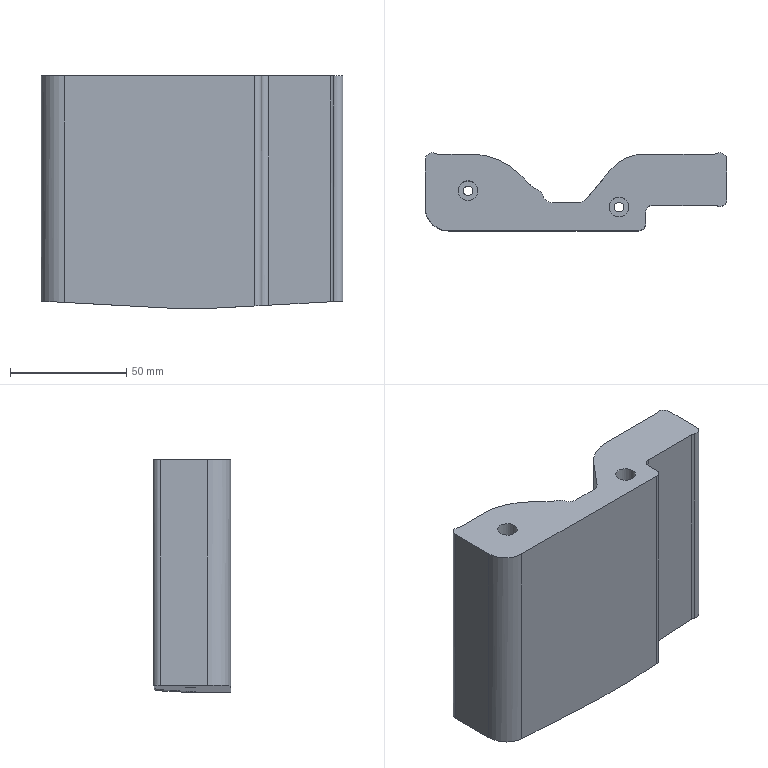Part | STEP file | lll_id246_x_t | 1 solid | 35 faces | box 130 x 33.5 x 100 mm | volume 301395 mm3 | cylinder 19 | plane 16 | commonest cylinder face diameters 6 x8 8 x3 4.2 x2 8.5 x2 20 x1 38 x1
STEP:
#1=CARTESIAN_POINT('',(386.218,20.929,-7.5));
#2=VERTEX_POINT('',#1);
#3=CARTESIAN_POINT('',(383.154,19.5,-7.5));
#4=VERTEX_POINT('',#3);
#5=CARTESIAN_POINT('',(383.154,23.5,-7.5));
#6=DIRECTION('',(0.,0.,-1.));
#7=DIRECTION('',(-1.,0.,0.));
#8=AXIS2_PLACEMENT_3D('',#5,#6,#7);
#9=CIRCLE('',#8,4.);
#10=EDGE_CURVE('',#2,#4,#9,.T.);
#11=ORIENTED_EDGE('',*,*,#10,.F.);
#12=CARTESIAN_POINT('',(392.,27.82,-7.5));
#13=VERTEX_POINT('',#12);
#14=CARTESIAN_POINT('',(562.911,231.504,-7.5));
#15=DIRECTION('',(0.6428,0.766,0.));
#16=VECTOR('',#15,1.);
#17=LINE('',#14,#16);
#18=EDGE_CURVE('',#2,#13,#17,.T.);
#19=ORIENTED_EDGE('',*,*,#18,.T.);
#20=CARTESIAN_POINT('',(392.,7.5,-7.5));
#21=VERTEX_POINT('',#20);
#22=CARTESIAN_POINT('',(392.,48.5,-7.5));
#23=DIRECTION('',(0.,-1.,0.));
#24=VECTOR('',#23,1.);
#25=LINE('',#22,#24);
#26=EDGE_CURVE('',#13,#21,#25,.T.);
#27=ORIENTED_EDGE('',*,*,#26,.T.);
#28=CARTESIAN_POINT('',(372.,7.5,-7.5));
#29=VERTEX_POINT('',#28);
#30=CARTESIAN_POINT('',(781.007,7.5,-7.5));
#31=DIRECTION('',(1.,0.,0.));
#32=VECTOR('',#31,1.);
#33=LINE('',#30,#32);
#34=EDGE_CURVE('',#29,#21,#33,.T.);
#35=ORIENTED_EDGE('',*,*,#34,.F.);
#36=CARTESIAN_POINT('',(372.,19.5,-7.5));
#37=VERTEX_POINT('',#36);
#38=CARTESIAN_POINT('',(372.,7.5,-7.5));
#39=DIRECTION('',(0.,-1.,0.));
#40=VECTOR('',#39,1.);
#41=LINE('',#38,#40);
#42=EDGE_CURVE('',#37,#29,#41,.T.);
#43=ORIENTED_EDGE('',*,*,#42,.F.);
#44=CARTESIAN_POINT('',(781.007,19.5,-7.5));
#45=DIRECTION('',(-1.,0.,0.));
#46=VECTOR('',#45,1.);
#47=LINE('',#44,#46);
#48=EDGE_CURVE('',#4,#37,#47,.T.);
#49=ORIENTED_EDGE('',*,*,#48,.F.);
#50=EDGE_LOOP('',(#11,#19,#27,#35,#43,#49));
#51=FACE_OUTER_BOUND('',#50,.T.);
#52=CARTESIAN_POINT('',(781.007,48.5,-7.5));
#53=DIRECTION('',(0.,0.,-1.));
#54=DIRECTION('',(1.,0.,0.));
#55=AXIS2_PLACEMENT_3D('',#52,#53,#54);
#56=PLANE('',#55);
#57=ADVANCED_FACE('',(#51),#56,.T.);
#58=CARTESIAN_POINT('',(331.25,24.75,92.5));
#59=VERTEX_POINT('',#58);
#60=CARTESIAN_POINT('',(335.5,24.75,92.5));
#61=DIRECTION('',(0.,0.,1.));
#62=DIRECTION('',(-1.,0.,0.));
#63=AXIS2_PLACEMENT_3D('',#60,#61,#62);
#64=CIRCLE('',#63,4.25);
#65=EDGE_CURVE('',#59,#59,#64,.T.);
#66=ORIENTED_EDGE('',*,*,#65,.F.);
#67=EDGE_LOOP('',(#66));
#68=FACE_BOUND('',#67,.T.);
#69=CARTESIAN_POINT('',(396.25,17.75,92.5));
#70=VERTEX_POINT('',#69);
#71=CARTESIAN_POINT('',(400.5,17.75,92.5));
#72=DIRECTION('',(0.,0.,-1.));
#73=DIRECTION('',(-1.,0.,0.));
#74=AXIS2_PLACEMENT_3D('',#71,#72,#73);
#75=CIRCLE('',#74,4.25);
#76=EDGE_CURVE('',#70,#70,#75,.T.);
#77=ORIENTED_EDGE('',*,*,#76,.T.);
#78=EDGE_LOOP('',(#77));
#79=FACE_BOUND('',#78,.T.);
#80=CARTESIAN_POINT('',(441.602,40.5,92.5));
#81=VERTEX_POINT('',#80);
#82=CARTESIAN_POINT('',(411.5,40.5,92.5));
#83=VERTEX_POINT('',#82);
#84=CARTESIAN_POINT('',(444.,40.5,92.5));
#85=DIRECTION('',(-1.,0.,0.));
#86=VECTOR('',#85,1.);
#87=LINE('',#84,#86);
#88=EDGE_CURVE('',#81,#83,#87,.T.);
#89=ORIENTED_EDGE('',*,*,#88,.T.);
#90=CARTESIAN_POINT('',(396.945,33.713,92.5));
#91=VERTEX_POINT('',#90);
#92=CARTESIAN_POINT('',(411.5,21.5,92.5));
#93=DIRECTION('',(0.,0.,1.));
#94=DIRECTION('',(-1.,0.,0.));
#95=AXIS2_PLACEMENT_3D('',#92,#93,#94);
#96=CIRCLE('',#95,19.);
#97=EDGE_CURVE('',#83,#91,#96,.T.);
#98=ORIENTED_EDGE('',*,*,#97,.T.);
#99=CARTESIAN_POINT('',(386.218,20.929,92.5));
#100=VERTEX_POINT('',#99);
#101=CARTESIAN_POINT('',(410.127,49.423,92.5));
#102=DIRECTION('',(0.6428,0.766,0.));
#103=VECTOR('',#102,1.);
#104=LINE('',#101,#103);
#105=EDGE_CURVE('',#100,#91,#104,.T.);
#106=ORIENTED_EDGE('',*,*,#105,.F.);
#107=CARTESIAN_POINT('',(383.154,19.5,92.5));
#108=VERTEX_POINT('',#107);
#109=CARTESIAN_POINT('',(383.154,23.5,92.5));
#110=DIRECTION('',(0.,0.,-1.));
#111=DIRECTION('',(-1.,0.,0.));
#112=AXIS2_PLACEMENT_3D('',#109,#110,#111);
#113=CIRCLE('',#112,4.);
#114=EDGE_CURVE('',#100,#108,#113,.T.);
#115=ORIENTED_EDGE('',*,*,#114,.T.);
#116=CARTESIAN_POINT('',(371.697,19.5,92.5));
#117=VERTEX_POINT('',#116);
#118=CARTESIAN_POINT('',(444.,19.5,92.5));
#119=DIRECTION('',(1.,0.,0.));
#120=VECTOR('',#119,1.);
#121=LINE('',#118,#120);
#122=EDGE_CURVE('',#117,#108,#121,.T.);
#123=ORIENTED_EDGE('',*,*,#122,.F.);
#124=CARTESIAN_POINT('',(367.848,22.409,92.5));
#125=VERTEX_POINT('',#124);
#126=CARTESIAN_POINT('',(371.697,23.5,92.5));
#127=DIRECTION('',(0.,0.,1.));
#128=DIRECTION('',(-1.,0.,0.));
#129=AXIS2_PLACEMENT_3D('',#126,#127,#128);
#130=CIRCLE('',#129,4.);
#131=EDGE_CURVE('',#125,#117,#130,.T.);
#132=ORIENTED_EDGE('',*,*,#131,.F.);
#133=CARTESIAN_POINT('',(365.881,24.849,92.5));
#134=VERTEX_POINT('',#133);
#135=CARTESIAN_POINT('',(364.,21.318,92.5));
#136=DIRECTION('',(0.,0.,-1.));
#137=DIRECTION('',(-1.,0.,0.));
#138=AXIS2_PLACEMENT_3D('',#135,#136,#137);
#139=CIRCLE('',#138,4.);
#140=EDGE_CURVE('',#134,#125,#139,.T.);
#141=ORIENTED_EDGE('',*,*,#140,.F.);
#142=CARTESIAN_POINT('',(361.142,28.358,92.5));
#143=VERTEX_POINT('',#142);
#144=CARTESIAN_POINT('',(375.216,42.407,92.5));
#145=DIRECTION('',(0.,0.,1.));
#146=DIRECTION('',(-1.,0.,0.));
#147=AXIS2_PLACEMENT_3D('',#144,#145,#146);
#148=CIRCLE('',#147,19.886);
#149=EDGE_CURVE('',#143,#134,#148,.T.);
#150=ORIENTED_EDGE('',*,*,#149,.F.);
#151=CARTESIAN_POINT('',(357.787,31.713,92.5));
#152=VERTEX_POINT('',#151);
#153=CARTESIAN_POINT('',(406.25,-16.75,92.5));
#154=DIRECTION('',(0.7071,-0.7071,0.));
#155=VECTOR('',#154,1.);
#156=LINE('',#153,#155);
#157=EDGE_CURVE('',#152,#143,#156,.T.);
#158=ORIENTED_EDGE('',*,*,#157,.F.);
#159=CARTESIAN_POINT('',(336.574,40.5,92.5));
#160=VERTEX_POINT('',#159);
#161=CARTESIAN_POINT('',(336.574,10.502,92.5));
#162=DIRECTION('',(0.,0.,-1.));
#163=DIRECTION('',(-1.,0.,0.));
#164=AXIS2_PLACEMENT_3D('',#161,#162,#163);
#165=CIRCLE('',#164,29.998);
#166=EDGE_CURVE('',#160,#152,#165,.T.);
#167=ORIENTED_EDGE('',*,*,#166,.F.);
#168=CARTESIAN_POINT('',(322.398,40.5,92.5));
#169=VERTEX_POINT('',#168);
#170=CARTESIAN_POINT('',(444.,40.5,92.5));
#171=DIRECTION('',(-1.,0.,0.));
#172=VECTOR('',#171,1.);
#173=LINE('',#170,#172);
#174=EDGE_CURVE('',#160,#169,#173,.T.);
#175=ORIENTED_EDGE('',*,*,#174,.T.);
#176=CARTESIAN_POINT('',(321.199,40.75,92.5));
#177=VERTEX_POINT('',#176);
#178=CARTESIAN_POINT('',(322.398,43.5,92.5));
#179=DIRECTION('',(0.,0.,1.));
#180=DIRECTION('',(-1.,0.,0.));
#181=AXIS2_PLACEMENT_3D('',#178,#179,#180);
#182=CIRCLE('',#181,3.);
#183=EDGE_CURVE('',#177,#169,#182,.T.);
#184=ORIENTED_EDGE('',*,*,#183,.F.);
#185=CARTESIAN_POINT('',(317.,38.,92.5));
#186=VERTEX_POINT('',#185);
#187=CARTESIAN_POINT('',(320.,38.,92.5));
#188=DIRECTION('',(0.,0.,1.));
#189=DIRECTION('',(-1.,0.,0.));
#190=AXIS2_PLACEMENT_3D('',#187,#188,#189);
#191=CIRCLE('',#190,3.);
#192=EDGE_CURVE('',#177,#186,#191,.T.);
#193=ORIENTED_EDGE('',*,*,#192,.T.);
#194=CARTESIAN_POINT('',(317.,17.5,92.5));
#195=VERTEX_POINT('',#194);
#196=CARTESIAN_POINT('',(317.,21.,92.5));
#197=DIRECTION('',(0.,1.,0.));
#198=VECTOR('',#197,1.);
#199=LINE('',#196,#198);
#200=EDGE_CURVE('',#195,#186,#199,.T.);
#201=ORIENTED_EDGE('',*,*,#200,.F.);
#202=CARTESIAN_POINT('',(327.,7.5,92.5));
#203=VERTEX_POINT('',#202);
#204=CARTESIAN_POINT('',(327.,17.5,92.5));
#205=DIRECTION('',(0.,0.,1.));
#206=DIRECTION('',(-1.,0.,0.));
#207=AXIS2_PLACEMENT_3D('',#204,#205,#206);
#208=CIRCLE('',#207,10.);
#209=EDGE_CURVE('',#195,#203,#208,.T.);
#210=ORIENTED_EDGE('',*,*,#209,.T.);
#211=CARTESIAN_POINT('',(409.,7.5,92.5));
#212=VERTEX_POINT('',#211);
#213=CARTESIAN_POINT('',(444.,7.5,92.5));
#214=DIRECTION('',(1.,0.,0.));
#215=VECTOR('',#214,1.);
#216=LINE('',#213,#215);
#217=EDGE_CURVE('',#203,#212,#216,.T.);
#218=ORIENTED_EDGE('',*,*,#217,.T.);
#219=CARTESIAN_POINT('',(412.,10.5,92.5));
#220=VERTEX_POINT('',#219);
#221=CARTESIAN_POINT('',(409.,10.5,92.5));
#222=DIRECTION('',(0.,0.,1.));
#223=DIRECTION('',(-1.,0.,0.));
#224=AXIS2_PLACEMENT_3D('',#221,#222,#223);
#225=CIRCLE('',#224,3.);
#226=EDGE_CURVE('',#212,#220,#225,.T.);
#227=ORIENTED_EDGE('',*,*,#226,.T.);
#228=CARTESIAN_POINT('',(412.,15.5,92.5));
#229=VERTEX_POINT('',#228);
#230=CARTESIAN_POINT('',(412.,21.,92.5));
#231=DIRECTION('',(0.,1.,0.));
#232=VECTOR('',#231,1.);
#233=LINE('',#230,#232);
#234=EDGE_CURVE('',#220,#229,#233,.T.);
#235=ORIENTED_EDGE('',*,*,#234,.T.);
#236=CARTESIAN_POINT('',(415.,18.5,92.5));
#237=VERTEX_POINT('',#236);
#238=CARTESIAN_POINT('',(415.,15.5,92.5));
#239=DIRECTION('',(0.,0.,1.));
#240=DIRECTION('',(-1.,0.,0.));
#241=AXIS2_PLACEMENT_3D('',#238,#239,#240);
#242=CIRCLE('',#241,3.);
#243=EDGE_CURVE('',#237,#229,#242,.T.);
#244=ORIENTED_EDGE('',*,*,#243,.F.);
#245=CARTESIAN_POINT('',(441.602,18.5,92.5));
#246=VERTEX_POINT('',#245);
#247=CARTESIAN_POINT('',(444.,18.5,92.5));
#248=DIRECTION('',(-1.,0.,0.));
#249=VECTOR('',#248,1.);
#250=LINE('',#247,#249);
#251=EDGE_CURVE('',#246,#237,#250,.T.);
#252=ORIENTED_EDGE('',*,*,#251,.F.);
#253=CARTESIAN_POINT('',(442.801,18.25,92.5));
#254=VERTEX_POINT('',#253);
#255=CARTESIAN_POINT('',(441.602,15.5,92.5));
#256=DIRECTION('',(0.,0.,-1.));
#257=DIRECTION('',(-1.,0.,0.));
#258=AXIS2_PLACEMENT_3D('',#255,#256,#257);
#259=CIRCLE('',#258,3.);
#260=EDGE_CURVE('',#246,#254,#259,.T.);
#261=ORIENTED_EDGE('',*,*,#260,.T.);
#262=CARTESIAN_POINT('',(447.,21.,92.5));
#263=VERTEX_POINT('',#262);
#264=CARTESIAN_POINT('',(444.,21.,92.5));
#265=DIRECTION('',(0.,0.,-1.));
#266=DIRECTION('',(-1.,0.,0.));
#267=AXIS2_PLACEMENT_3D('',#264,#265,#266);
#268=CIRCLE('',#267,3.);
#269=EDGE_CURVE('',#263,#254,#268,.T.);
#270=ORIENTED_EDGE('',*,*,#269,.F.);
#271=CARTESIAN_POINT('',(447.,38.,92.5));
#272=VERTEX_POINT('',#271);
#273=CARTESIAN_POINT('',(447.,21.,92.5));
#274=DIRECTION('',(0.,-1.,0.));
#275=VECTOR('',#274,1.);
#276=LINE('',#273,#275);
#277=EDGE_CURVE('',#272,#263,#276,.T.);
#278=ORIENTED_EDGE('',*,*,#277,.F.);
#279=CARTESIAN_POINT('',(442.801,40.75,92.5));
#280=VERTEX_POINT('',#279);
#281=CARTESIAN_POINT('',(444.,38.,92.5));
#282=DIRECTION('',(0.,0.,1.));
#283=DIRECTION('',(-1.,0.,0.));
#284=AXIS2_PLACEMENT_3D('',#281,#282,#283);
#285=CIRCLE('',#284,3.);
#286=EDGE_CURVE('',#272,#280,#285,.T.);
#287=ORIENTED_EDGE('',*,*,#286,.T.);
#288=CARTESIAN_POINT('',(441.602,43.5,92.5));
#289=DIRECTION('',(0.,0.,-1.));
#290=DIRECTION('',(-1.,0.,0.));
#291=AXIS2_PLACEMENT_3D('',#288,#289,#290);
#292=CIRCLE('',#291,3.);
#293=EDGE_CURVE('',#280,#81,#292,.T.);
#294=ORIENTED_EDGE('',*,*,#293,.T.);
#295=EDGE_LOOP('',(#89,#98,#106,#115,#123,#132,#141,#150,#158,#167,#175,#184,#193,#201,#210,#218,#227,#235,#244,#252,#261,#270,#278,#287,#294));
#296=FACE_BOUND('',#295,.T.);
#297=CARTESIAN_POINT('',(444.,21.,92.5));
#298=DIRECTION('',(0.,0.,-1.));
#299=DIRECTION('',(1.,0.,0.));
#300=AXIS2_PLACEMENT_3D('',#297,#298,#299);
#301=PLANE('',#300);
#302=ADVANCED_FACE('',(#68,#79,#296),#301,.F.);
#303=CARTESIAN_POINT('',(337.6,24.75,-5.624));
#304=VERTEX_POINT('',#303);
#305=CARTESIAN_POINT('',(335.5,24.75,-5.509));
#306=DIRECTION('',(0.05446,0.,0.9985));
#307=DIRECTION('',(0.9985,0.,-0.05446));
#308=AXIS2_PLACEMENT_3D('',#305,#306,#307);
#309=ELLIPSE('',#308,2.103,2.1);
#310=EDGE_CURVE('',#304,#304,#309,.T.);
#311=ORIENTED_EDGE('',*,*,#310,.T.);
#312=EDGE_LOOP('',(#311));
#313=FACE_BOUND('',#312,.T.);
#314=CARTESIAN_POINT('',(371.697,19.5,-7.483));
#315=VERTEX_POINT('',#314);
#316=CARTESIAN_POINT('',(367.848,22.409,-7.274));
#317=VERTEX_POINT('',#316);
#318=CARTESIAN_POINT('',(371.697,23.5,-7.483));
#319=DIRECTION('',(-0.05446,0.,-0.9985));
#320=DIRECTION('',(-0.9985,0.,0.05446));
#321=AXIS2_PLACEMENT_3D('',#318,#319,#320);
#322=ELLIPSE('',#321,4.006,4.);
#323=EDGE_CURVE('',#315,#317,#322,.T.);
#324=ORIENTED_EDGE('',*,*,#323,.F.);
#325=CARTESIAN_POINT('',(317.,19.5,-4.5));
#326=DIRECTION('',(-0.9985,0.,0.05446));
#327=VECTOR('',#326,1.);
#328=LINE('',#325,#327);
#329=EDGE_CURVE('',#37,#315,#328,.T.);
#330=ORIENTED_EDGE('',*,*,#329,.F.);
#331=ORIENTED_EDGE('',*,*,#42,.T.);
#332=CARTESIAN_POINT('',(327.,7.5,-5.045));
#333=VERTEX_POINT('',#332);
#334=CARTESIAN_POINT('',(317.,7.5,-4.5));
#335=DIRECTION('',(-0.9985,0.,0.05446));
#336=VECTOR('',#335,1.);
#337=LINE('',#334,#336);
#338=EDGE_CURVE('',#29,#333,#337,.T.);
#339=ORIENTED_EDGE('',*,*,#338,.T.);
#340=CARTESIAN_POINT('',(317.,17.5,-4.5));
#341=VERTEX_POINT('',#340);
#342=CARTESIAN_POINT('',(327.,17.5,-5.045));
#343=DIRECTION('',(-0.05446,0.,-0.9985));
#344=DIRECTION('',(-0.9985,0.,0.05446));
#345=AXIS2_PLACEMENT_3D('',#342,#343,#344);
#346=ELLIPSE('',#345,10.015,10.);
#347=EDGE_CURVE('',#333,#341,#346,.T.);
#348=ORIENTED_EDGE('',*,*,#347,.T.);
#349=CARTESIAN_POINT('',(317.,38.,-4.5));
#350=VERTEX_POINT('',#349);
#351=CARTESIAN_POINT('',(317.,7.5,-4.5));
#352=DIRECTION('',(0.,-1.,0.));
#353=VECTOR('',#352,1.);
#354=LINE('',#351,#353);
#355=EDGE_CURVE('',#350,#341,#354,.T.);
#356=ORIENTED_EDGE('',*,*,#355,.F.);
#357=CARTESIAN_POINT('',(321.199,40.75,-4.729));
#358=VERTEX_POINT('',#357);
#359=CARTESIAN_POINT('',(320.,38.,-4.664));
#360=DIRECTION('',(0.05446,0.,0.9985));
#361=DIRECTION('',(-0.9985,0.,0.05446));
#362=AXIS2_PLACEMENT_3D('',#359,#360,#361);
#363=ELLIPSE('',#362,3.004,3.);
#364=EDGE_CURVE('',#358,#350,#363,.T.);
#365=ORIENTED_EDGE('',*,*,#364,.F.);
#366=CARTESIAN_POINT('',(322.398,40.5,-4.794));
#367=VERTEX_POINT('',#366);
#368=CARTESIAN_POINT('',(322.398,43.5,-4.794));
#369=DIRECTION('',(0.05446,0.,0.9985));
#370=DIRECTION('',(-0.9985,0.,0.05446));
#371=AXIS2_PLACEMENT_3D('',#368,#369,#370);
#372=ELLIPSE('',#371,3.004,3.);
#373=EDGE_CURVE('',#358,#367,#372,.T.);
#374=ORIENTED_EDGE('',*,*,#373,.T.);
#375=CARTESIAN_POINT('',(336.574,40.5,-5.568));
#376=VERTEX_POINT('',#375);
#377=CARTESIAN_POINT('',(317.,40.5,-4.5));
#378=DIRECTION('',(0.9985,0.,-0.05446));
#379=VECTOR('',#378,1.);
#380=LINE('',#377,#379);
#381=EDGE_CURVE('',#367,#376,#380,.T.);
#382=ORIENTED_EDGE('',*,*,#381,.T.);
#383=CARTESIAN_POINT('',(357.787,31.713,-6.725));
#384=VERTEX_POINT('',#383);
#385=CARTESIAN_POINT('',(336.574,10.502,-5.568));
#386=DIRECTION('',(-0.05446,0.,-0.9985));
#387=DIRECTION('',(-0.9985,0.,0.05446));
#388=AXIS2_PLACEMENT_3D('',#385,#386,#387);
#389=ELLIPSE('',#388,30.042,29.998);
#390=EDGE_CURVE('',#376,#384,#389,.T.);
#391=ORIENTED_EDGE('',*,*,#390,.T.);
#392=CARTESIAN_POINT('',(361.142,28.358,-6.908));
#393=VERTEX_POINT('',#392);
#394=CARTESIAN_POINT('',(349.452,40.048,-6.27));
#395=DIRECTION('',(-0.7066,0.7066,0.03854));
#396=VECTOR('',#395,1.);
#397=LINE('',#394,#396);
#398=EDGE_CURVE('',#393,#384,#397,.T.);
#399=ORIENTED_EDGE('',*,*,#398,.F.);
#400=CARTESIAN_POINT('',(365.881,24.849,-7.166));
#401=VERTEX_POINT('',#400);
#402=CARTESIAN_POINT('',(375.216,42.407,-7.675));
#403=DIRECTION('',(-0.05446,0.,-0.9985));
#404=DIRECTION('',(-0.9985,0.,0.05446));
#405=AXIS2_PLACEMENT_3D('',#402,#403,#404);
#406=ELLIPSE('',#405,19.915,19.886);
#407=EDGE_CURVE('',#401,#393,#406,.T.);
#408=ORIENTED_EDGE('',*,*,#407,.F.);
#409=CARTESIAN_POINT('',(364.,21.318,-7.064));
#410=DIRECTION('',(0.05446,0.,0.9985));
#411=DIRECTION('',(-0.9985,0.,0.05446));
#412=AXIS2_PLACEMENT_3D('',#409,#410,#411);
#413=ELLIPSE('',#412,4.006,4.);
#414=EDGE_CURVE('',#317,#401,#413,.T.);
#415=ORIENTED_EDGE('',*,*,#414,.F.);
#416=EDGE_LOOP('',(#324,#330,#331,#339,#348,#356,#365,#374,#382,#391,#399,#408,#415));
#417=FACE_BOUND('',#416,.T.);
#418=CARTESIAN_POINT('',(317.,7.5,-4.5));
#419=DIRECTION('',(-0.05446,0.,-0.9985));
#420=DIRECTION('',(0.9985,0.,-0.05446));
#421=AXIS2_PLACEMENT_3D('',#418,#419,#420);
#422=PLANE('',#421);
#423=ADVANCED_FACE('',(#313,#417),#422,.T.);
#424=CARTESIAN_POINT('',(398.4,17.75,-7.151));
#425=VERTEX_POINT('',#424);
#426=CARTESIAN_POINT('',(400.5,17.75,-7.036));
#427=DIRECTION('',(0.05446,0.,-0.9985));
#428=DIRECTION('',(-0.9985,0.,-0.05446));
#429=AXIS2_PLACEMENT_3D('',#426,#427,#428);
#430=ELLIPSE('',#429,2.103,2.1);
#431=EDGE_CURVE('',#425,#425,#430,.T.);
#432=ORIENTED_EDGE('',*,*,#431,.F.);
#433=EDGE_LOOP('',(#432));
#434=FACE_BOUND('',#433,.T.);
#435=CARTESIAN_POINT('',(396.945,33.713,-7.23));
#436=VERTEX_POINT('',#435);
#437=CARTESIAN_POINT('',(404.771,43.04,-6.803));
#438=DIRECTION('',(-0.6424,-0.7656,-0.03504));
#439=VECTOR('',#438,1.);
#440=LINE('',#437,#439);
#441=EDGE_CURVE('',#436,#13,#440,.T.);
#442=ORIENTED_EDGE('',*,*,#441,.F.);
#443=CARTESIAN_POINT('',(411.5,40.5,-6.436));
#444=VERTEX_POINT('',#443);
#445=CARTESIAN_POINT('',(411.5,21.5,-6.436));
#446=DIRECTION('',(-0.05446,0.,0.9985));
#447=DIRECTION('',(0.9985,0.,0.05446));
#448=AXIS2_PLACEMENT_3D('',#445,#446,#447);
#449=ELLIPSE('',#448,19.028,19.);
#450=EDGE_CURVE('',#444,#436,#449,.T.);
#451=ORIENTED_EDGE('',*,*,#450,.F.);
#452=CARTESIAN_POINT('',(441.602,40.5,-4.794));
#453=VERTEX_POINT('',#452);
#454=CARTESIAN_POINT('',(447.,40.5,-4.5));
#455=DIRECTION('',(0.9985,0.,0.05446));
#456=VECTOR('',#455,1.);
#457=LINE('',#454,#456);
#458=EDGE_CURVE('',#444,#453,#457,.T.);
#459=ORIENTED_EDGE('',*,*,#458,.T.);
#460=CARTESIAN_POINT('',(442.801,40.75,-4.729));
#461=VERTEX_POINT('',#460);
#462=CARTESIAN_POINT('',(441.602,43.5,-4.794));
#463=DIRECTION('',(-0.05446,0.,0.9985));
#464=DIRECTION('',(0.9985,0.,0.05446));
#465=AXIS2_PLACEMENT_3D('',#462,#463,#464);
#466=ELLIPSE('',#465,3.004,3.);
#467=EDGE_CURVE('',#453,#461,#466,.T.);
#468=ORIENTED_EDGE('',*,*,#467,.T.);
#469=CARTESIAN_POINT('',(447.,38.,-4.5));
#470=VERTEX_POINT('',#469);
#471=CARTESIAN_POINT('',(444.,38.,-4.664));
#472=DIRECTION('',(-0.05446,0.,0.9985));
#473=DIRECTION('',(0.9985,0.,0.05446));
#474=AXIS2_PLACEMENT_3D('',#471,#472,#473);
#475=ELLIPSE('',#474,3.004,3.);
#476=EDGE_CURVE('',#470,#461,#475,.T.);
#477=ORIENTED_EDGE('',*,*,#476,.F.);
#478=CARTESIAN_POINT('',(447.,21.,-4.5));
#479=VERTEX_POINT('',#478);
#480=CARTESIAN_POINT('',(447.,7.5,-4.5));
#481=DIRECTION('',(0.,-1.,0.));
#482=VECTOR('',#481,1.);
#483=LINE('',#480,#482);
#484=EDGE_CURVE('',#470,#479,#483,.T.);
#485=ORIENTED_EDGE('',*,*,#484,.T.);
#486=CARTESIAN_POINT('',(442.801,18.25,-4.729));
#487=VERTEX_POINT('',#486);
#488=CARTESIAN_POINT('',(444.,21.,-4.664));
#489=DIRECTION('',(0.05446,0.,-0.9985));
#490=DIRECTION('',(0.9985,0.,0.05446));
#491=AXIS2_PLACEMENT_3D('',#488,#489,#490);
#492=ELLIPSE('',#491,3.004,3.);
#493=EDGE_CURVE('',#479,#487,#492,.T.);
#494=ORIENTED_EDGE('',*,*,#493,.T.);
#495=CARTESIAN_POINT('',(441.602,18.5,-4.794));
#496=VERTEX_POINT('',#495);
#497=CARTESIAN_POINT('',(441.602,15.5,-4.794));
#498=DIRECTION('',(0.05446,0.,-0.9985));
#499=DIRECTION('',(0.9985,0.,0.05446));
#500=AXIS2_PLACEMENT_3D('',#497,#498,#499);
#501=ELLIPSE('',#500,3.004,3.);
#502=EDGE_CURVE('',#496,#487,#501,.T.);
#503=ORIENTED_EDGE('',*,*,#502,.F.);
#504=CARTESIAN_POINT('',(415.,18.5,-6.245));
#505=VERTEX_POINT('',#504);
#506=CARTESIAN_POINT('',(447.,18.5,-4.5));
#507=DIRECTION('',(-0.9985,0.,-0.05446));
#508=VECTOR('',#507,1.);
#509=LINE('',#506,#508);
#510=EDGE_CURVE('',#496,#505,#509,.T.);
#511=ORIENTED_EDGE('',*,*,#510,.T.);
#512=CARTESIAN_POINT('',(412.,15.5,-6.409));
#513=VERTEX_POINT('',#512);
#514=CARTESIAN_POINT('',(415.,15.5,-6.245));
#515=DIRECTION('',(0.05446,0.,-0.9985));
#516=DIRECTION('',(0.9985,0.,0.05446));
#517=AXIS2_PLACEMENT_3D('',#514,#515,#516);
#518=ELLIPSE('',#517,3.004,3.);
#519=EDGE_CURVE('',#513,#505,#518,.T.);
#520=ORIENTED_EDGE('',*,*,#519,.F.);
#521=CARTESIAN_POINT('',(412.,10.5,-6.409));
#522=VERTEX_POINT('',#521);
#523=CARTESIAN_POINT('',(412.,7.5,-6.409));
#524=DIRECTION('',(0.,-1.,0.));
#525=VECTOR('',#524,1.);
#526=LINE('',#523,#525);
#527=EDGE_CURVE('',#513,#522,#526,.T.);
#528=ORIENTED_EDGE('',*,*,#527,.T.);
#529=CARTESIAN_POINT('',(409.,7.5,-6.573));
#530=VERTEX_POINT('',#529);
#531=CARTESIAN_POINT('',(409.,10.5,-6.573));
#532=DIRECTION('',(-0.05446,0.,0.9985));
#533=DIRECTION('',(0.9985,0.,0.05446));
#534=AXIS2_PLACEMENT_3D('',#531,#532,#533);
#535=ELLIPSE('',#534,3.004,3.);
#536=EDGE_CURVE('',#530,#522,#535,.T.);
#537=ORIENTED_EDGE('',*,*,#536,.F.);
#538=CARTESIAN_POINT('',(447.,7.5,-4.5));
#539=DIRECTION('',(-0.9985,0.,-0.05446));
#540=VECTOR('',#539,1.);
#541=LINE('',#538,#540);
#542=EDGE_CURVE('',#530,#21,#541,.T.);
#543=ORIENTED_EDGE('',*,*,#542,.T.);
#544=ORIENTED_EDGE('',*,*,#26,.F.);
#545=EDGE_LOOP('',(#442,#451,#459,#468,#477,#485,#494,#503,#511,#520,#528,#537,#543,#544));
#546=FACE_BOUND('',#545,.T.);
#547=CARTESIAN_POINT('',(447.,7.5,-4.5));
#548=DIRECTION('',(-0.05446,0.,0.9985));
#549=DIRECTION('',(-0.9985,0.,-0.05446));
#550=AXIS2_PLACEMENT_3D('',#547,#548,#549);
#551=PLANE('',#550);
#552=ADVANCED_FACE('',(#434,#546),#551,.F.);
#553=CARTESIAN_POINT('',(333.4,24.75,30.747));
#554=VERTEX_POINT('',#553);
#555=CARTESIAN_POINT('',(335.5,24.75,30.747));
#556=DIRECTION('',(0.,0.,-1.));
#557=DIRECTION('',(-1.,0.,0.));
#558=AXIS2_PLACEMENT_3D('',#555,#556,#557);
#559=CIRCLE('',#558,2.1);
#560=EDGE_CURVE('',#554,#554,#559,.T.);
#561=ORIENTED_EDGE('',*,*,#560,.F.);
#562=EDGE_LOOP('',(#561));
#563=FACE_BOUND('',#562,.T.);
#564=ORIENTED_EDGE('',*,*,#310,.F.);
#565=EDGE_LOOP('',(#564));
#566=FACE_BOUND('',#565,.T.);
#567=CARTESIAN_POINT('',(335.5,24.75,30.747));
#568=DIRECTION('',(0.,0.,-1.));
#569=DIRECTION('',(1.,0.,0.));
#570=AXIS2_PLACEMENT_3D('',#567,#568,#569);
#571=CYLINDRICAL_SURFACE('',#570,2.1);
#572=ADVANCED_FACE('',(#563,#566),#571,.F.);
#573=CARTESIAN_POINT('',(398.4,17.75,30.747));
#574=VERTEX_POINT('',#573);
#575=CARTESIAN_POINT('',(400.5,17.75,30.747));
#576=DIRECTION('',(0.,0.,-1.));
#577=DIRECTION('',(-1.,0.,0.));
#578=AXIS2_PLACEMENT_3D('',#575,#576,#577);
#579=CIRCLE('',#578,2.1);
#580=EDGE_CURVE('',#574,#574,#579,.T.);
#581=ORIENTED_EDGE('',*,*,#580,.T.);
#582=EDGE_LOOP('',(#581));
#583=FACE_BOUND('',#582,.T.);
#584=CARTESIAN_POINT('',(396.25,17.75,30.747));
#585=VERTEX_POINT('',#584);
#586=CARTESIAN_POINT('',(400.5,17.75,30.747));
#587=DIRECTION('',(0.,0.,-1.));
#588=DIRECTION('',(-1.,0.,0.));
#589=AXIS2_PLACEMENT_3D('',#586,#587,#588);
#590=CIRCLE('',#589,4.25);
#591=EDGE_CURVE('',#585,#585,#590,.T.);
#592=ORIENTED_EDGE('',*,*,#591,.F.);
#593=EDGE_LOOP('',(#592));
#594=FACE_BOUND('',#593,.T.);
#595=CARTESIAN_POINT('',(335.5,24.75,30.747));
#596=DIRECTION('',(0.,0.,-1.));
#597=DIRECTION('',(1.,0.,0.));
#598=AXIS2_PLACEMENT_3D('',#595,#596,#597);
#599=PLANE('',#598);
#600=ADVANCED_FACE('',(#583,#594),#599,.F.);
#601=CARTESIAN_POINT('',(331.25,24.75,30.747));
#602=VERTEX_POINT('',#601);
#603=CARTESIAN_POINT('',(335.5,24.75,30.747));
#604=DIRECTION('',(0.,0.,1.));
#605=DIRECTION('',(-1.,0.,0.));
#606=AXIS2_PLACEMENT_3D('',#603,#604,#605);
#607=CIRCLE('',#606,4.25);
#608=EDGE_CURVE('',#602,#602,#607,.T.);
#609=ORIENTED_EDGE('',*,*,#608,.T.);
#610=EDGE_LOOP('',(#609));
#611=FACE_BOUND('',#610,.T.);
#612=ORIENTED_EDGE('',*,*,#560,.T.);
#613=EDGE_LOOP('',(#612));
#614=FACE_BOUND('',#613,.T.);
#615=CARTESIAN_POINT('',(335.5,24.75,30.747));
#616=DIRECTION('',(0.,0.,-1.));
#617=DIRECTION('',(1.,0.,0.));
#618=AXIS2_PLACEMENT_3D('',#615,#616,#617);
#619=PLANE('',#618);
#620=ADVANCED_FACE('',(#611,#614),#619,.F.);
#621=ORIENTED_EDGE('',*,*,#431,.T.);
#622=EDGE_LOOP('',(#621));
#623=FACE_BOUND('',#622,.T.);
#624=ORIENTED_EDGE('',*,*,#580,.F.);
#625=EDGE_LOOP('',(#624));
#626=FACE_BOUND('',#625,.T.);
#627=CARTESIAN_POINT('',(400.5,17.75,30.747));
#628=DIRECTION('',(0.,0.,-1.));
#629=DIRECTION('',(1.,0.,0.));
#630=AXIS2_PLACEMENT_3D('',#627,#628,#629);
#631=CYLINDRICAL_SURFACE('',#630,2.1);
#632=ADVANCED_FACE('',(#623,#626),#631,.F.);
#633=ORIENTED_EDGE('',*,*,#608,.F.);
#634=EDGE_LOOP('',(#633));
#635=FACE_BOUND('',#634,.T.);
#636=ORIENTED_EDGE('',*,*,#65,.T.);
#637=EDGE_LOOP('',(#636));
#638=FACE_BOUND('',#637,.T.);
#639=CARTESIAN_POINT('',(335.5,24.75,240.747));
#640=DIRECTION('',(0.,0.,-1.));
#641=DIRECTION('',(1.,0.,0.));
#642=AXIS2_PLACEMENT_3D('',#639,#640,#641);
#643=CYLINDRICAL_SURFACE('',#642,4.25);
#644=ADVANCED_FACE('',(#635,#638),#643,.F.);
#645=ORIENTED_EDGE('',*,*,#591,.T.);
#646=EDGE_LOOP('',(#645));
#647=FACE_BOUND('',#646,.T.);
#648=ORIENTED_EDGE('',*,*,#76,.F.);
#649=EDGE_LOOP('',(#648));
#650=FACE_BOUND('',#649,.T.);
#651=CARTESIAN_POINT('',(400.5,17.75,240.747));
#652=DIRECTION('',(0.,0.,-1.));
#653=DIRECTION('',(1.,0.,0.));
#654=AXIS2_PLACEMENT_3D('',#651,#652,#653);
#655=CYLINDRICAL_SURFACE('',#654,4.25);
#656=ADVANCED_FACE('',(#647,#650),#655,.F.);
#657=ORIENTED_EDGE('',*,*,#10,.T.);
#658=CARTESIAN_POINT('',(383.154,19.5,-177.5));
#659=DIRECTION('',(0.,0.,1.));
#660=VECTOR('',#659,1.);
#661=LINE('',#658,#660);
#662=EDGE_CURVE('',#4,#108,#661,.T.);
#663=ORIENTED_EDGE('',*,*,#662,.T.);
#664=ORIENTED_EDGE('',*,*,#114,.F.);
#665=CARTESIAN_POINT('',(386.218,20.929,-177.5));
#666=DIRECTION('',(0.,0.,1.));
#667=VECTOR('',#666,1.);
#668=LINE('',#665,#667);
#669=EDGE_CURVE('',#2,#100,#668,.T.);
#670=ORIENTED_EDGE('',*,*,#669,.F.);
#671=EDGE_LOOP('',(#657,#663,#664,#670));
#672=FACE_OUTER_BOUND('',#671,.T.);
#673=CARTESIAN_POINT('',(383.154,23.5,-177.5));
#674=DIRECTION('',(0.,0.,1.));
#675=DIRECTION('',(1.,0.,0.));
#676=AXIS2_PLACEMENT_3D('',#673,#674,#675);
#677=CYLINDRICAL_SURFACE('',#676,4.);
#678=ADVANCED_FACE('',(#672),#677,.F.);
#679=CARTESIAN_POINT('',(371.697,19.5,-177.5));
#680=DIRECTION('',(0.,0.,1.));
#681=VECTOR('',#680,1.);
#682=LINE('',#679,#681);
#683=EDGE_CURVE('',#315,#117,#682,.T.);
#684=ORIENTED_EDGE('',*,*,#683,.T.);
#685=ORIENTED_EDGE('',*,*,#122,.T.);
#686=ORIENTED_EDGE('',*,*,#662,.F.);
#687=ORIENTED_EDGE('',*,*,#48,.T.);
#688=ORIENTED_EDGE('',*,*,#329,.T.);
#689=EDGE_LOOP('',(#684,#685,#686,#687,#688));
#690=FACE_OUTER_BOUND('',#689,.T.);
#691=CARTESIAN_POINT('',(383.154,19.5,-177.5));
#692=DIRECTION('',(0.,1.,0.));
#693=DIRECTION('',(-1.,0.,0.));
#694=AXIS2_PLACEMENT_3D('',#691,#692,#693);
#695=PLANE('',#694);
#696=ADVANCED_FACE('',(#690),#695,.T.);
#697=CARTESIAN_POINT('',(367.848,22.409,-177.5));
#698=DIRECTION('',(0.,0.,1.));
#699=VECTOR('',#698,1.);
#700=LINE('',#697,#699);
#701=EDGE_CURVE('',#317,#125,#700,.T.);
#702=ORIENTED_EDGE('',*,*,#701,.T.);
#703=ORIENTED_EDGE('',*,*,#131,.T.);
#704=ORIENTED_EDGE('',*,*,#683,.F.);
#705=ORIENTED_EDGE('',*,*,#323,.T.);
#706=EDGE_LOOP('',(#702,#703,#704,#705));
#707=FACE_OUTER_BOUND('',#706,.T.);
#708=CARTESIAN_POINT('',(371.697,23.5,-177.5));
#709=DIRECTION('',(0.,0.,1.));
#710=DIRECTION('',(1.,0.,0.));
#711=AXIS2_PLACEMENT_3D('',#708,#709,#710);
#712=CYLINDRICAL_SURFACE('',#711,4.);
#713=ADVANCED_FACE('',(#707),#712,.F.);
#714=CARTESIAN_POINT('',(365.881,24.849,-177.5));
#715=DIRECTION('',(0.,0.,1.));
#716=VECTOR('',#715,1.);
#717=LINE('',#714,#716);
#718=EDGE_CURVE('',#401,#134,#717,.T.);
#719=ORIENTED_EDGE('',*,*,#718,.T.);
#720=ORIENTED_EDGE('',*,*,#140,.T.);
#721=ORIENTED_EDGE('',*,*,#701,.F.);
#722=ORIENTED_EDGE('',*,*,#414,.T.);
#723=EDGE_LOOP('',(#719,#720,#721,#722));
#724=FACE_OUTER_BOUND('',#723,.T.);
#725=CARTESIAN_POINT('',(364.,21.318,-177.5));
#726=DIRECTION('',(0.,0.,1.));
#727=DIRECTION('',(1.,0.,0.));
#728=AXIS2_PLACEMENT_3D('',#725,#726,#727);
#729=CYLINDRICAL_SURFACE('',#728,4.);
#730=ADVANCED_FACE('',(#724),#729,.T.);
#731=CARTESIAN_POINT('',(361.142,28.358,-177.5));
#732=DIRECTION('',(0.,0.,1.));
#733=VECTOR('',#732,1.);
#734=LINE('',#731,#733);
#735=EDGE_CURVE('',#393,#143,#734,.T.);
#736=ORIENTED_EDGE('',*,*,#735,.T.);
#737=ORIENTED_EDGE('',*,*,#149,.T.);
#738=ORIENTED_EDGE('',*,*,#718,.F.);
#739=ORIENTED_EDGE('',*,*,#407,.T.);
#740=EDGE_LOOP('',(#736,#737,#738,#739));
#741=FACE_OUTER_BOUND('',#740,.T.);
#742=CARTESIAN_POINT('',(375.216,42.407,-177.5));
#743=DIRECTION('',(0.,0.,1.));
#744=DIRECTION('',(1.,0.,0.));
#745=AXIS2_PLACEMENT_3D('',#742,#743,#744);
#746=CYLINDRICAL_SURFACE('',#745,19.886);
#747=ADVANCED_FACE('',(#741),#746,.F.);
#748=CARTESIAN_POINT('',(357.787,31.713,-177.5));
#749=DIRECTION('',(0.,0.,1.));
#750=VECTOR('',#749,1.);
#751=LINE('',#748,#750);
#752=EDGE_CURVE('',#384,#152,#751,.T.);
#753=ORIENTED_EDGE('',*,*,#752,.T.);
#754=ORIENTED_EDGE('',*,*,#157,.T.);
#755=ORIENTED_EDGE('',*,*,#735,.F.);
#756=ORIENTED_EDGE('',*,*,#398,.T.);
#757=EDGE_LOOP('',(#753,#754,#755,#756));
#758=FACE_OUTER_BOUND('',#757,.T.);
#759=CARTESIAN_POINT('',(361.142,28.358,-177.5));
#760=DIRECTION('',(0.7071,0.7071,0.));
#761=DIRECTION('',(-0.7071,0.7071,0.));
#762=AXIS2_PLACEMENT_3D('',#759,#760,#761);
#763=PLANE('',#762);
#764=ADVANCED_FACE('',(#758),#763,.T.);
#765=CARTESIAN_POINT('',(336.574,40.5,-177.5));
#766=DIRECTION('',(0.,0.,1.));
#767=VECTOR('',#766,1.);
#768=LINE('',#765,#767);
#769=EDGE_CURVE('',#376,#160,#768,.T.);
#770=ORIENTED_EDGE('',*,*,#769,.T.);
#771=ORIENTED_EDGE('',*,*,#166,.T.);
#772=ORIENTED_EDGE('',*,*,#752,.F.);
#773=ORIENTED_EDGE('',*,*,#390,.F.);
#774=EDGE_LOOP('',(#770,#771,#772,#773));
#775=FACE_OUTER_BOUND('',#774,.T.);
#776=CARTESIAN_POINT('',(336.574,10.502,-177.5));
#777=DIRECTION('',(0.,0.,1.));
#778=DIRECTION('',(1.,0.,0.));
#779=AXIS2_PLACEMENT_3D('',#776,#777,#778);
#780=CYLINDRICAL_SURFACE('',#779,29.998);
#781=ADVANCED_FACE('',(#775),#780,.T.);
#782=CARTESIAN_POINT('',(322.398,40.5,-177.5));
#783=DIRECTION('',(0.,0.,1.));
#784=VECTOR('',#783,1.);
#785=LINE('',#782,#784);
#786=EDGE_CURVE('',#367,#169,#785,.T.);
#787=ORIENTED_EDGE('',*,*,#786,.T.);
#788=ORIENTED_EDGE('',*,*,#174,.F.);
#789=ORIENTED_EDGE('',*,*,#769,.F.);
#790=ORIENTED_EDGE('',*,*,#381,.F.);
#791=EDGE_LOOP('',(#787,#788,#789,#790));
#792=FACE_OUTER_BOUND('',#791,.T.);
#793=CARTESIAN_POINT('',(336.574,40.5,-177.5));
#794=DIRECTION('',(0.,1.,0.));
#795=DIRECTION('',(-1.,0.,0.));
#796=AXIS2_PLACEMENT_3D('',#793,#794,#795);
#797=PLANE('',#796);
#798=ADVANCED_FACE('',(#792),#797,.T.);
#799=CARTESIAN_POINT('',(321.199,40.75,-177.5));
#800=DIRECTION('',(0.,0.,1.));
#801=VECTOR('',#800,1.);
#802=LINE('',#799,#801);
#803=EDGE_CURVE('',#358,#177,#802,.T.);
#804=ORIENTED_EDGE('',*,*,#803,.T.);
#805=ORIENTED_EDGE('',*,*,#183,.T.);
#806=ORIENTED_EDGE('',*,*,#786,.F.);
#807=ORIENTED_EDGE('',*,*,#373,.F.);
#808=EDGE_LOOP('',(#804,#805,#806,#807));
#809=FACE_OUTER_BOUND('',#808,.T.);
#810=CARTESIAN_POINT('',(322.398,43.5,-177.5));
#811=DIRECTION('',(0.,0.,1.));
#812=DIRECTION('',(1.,0.,0.));
#813=AXIS2_PLACEMENT_3D('',#810,#811,#812);
#814=CYLINDRICAL_SURFACE('',#813,3.);
#815=ADVANCED_FACE('',(#809),#814,.F.);
#816=CARTESIAN_POINT('',(317.,38.,-177.5));
#817=DIRECTION('',(0.,0.,1.));
#818=VECTOR('',#817,1.);
#819=LINE('',#816,#818);
#820=EDGE_CURVE('',#350,#186,#819,.T.);
#821=ORIENTED_EDGE('',*,*,#820,.T.);
#822=ORIENTED_EDGE('',*,*,#192,.F.);
#823=ORIENTED_EDGE('',*,*,#803,.F.);
#824=ORIENTED_EDGE('',*,*,#364,.T.);
#825=EDGE_LOOP('',(#821,#822,#823,#824));
#826=FACE_OUTER_BOUND('',#825,.T.);
#827=CARTESIAN_POINT('',(320.,38.,-177.5));
#828=DIRECTION('',(0.,0.,1.));
#829=DIRECTION('',(1.,0.,0.));
#830=AXIS2_PLACEMENT_3D('',#827,#828,#829);
#831=CYLINDRICAL_SURFACE('',#830,3.);
#832=ADVANCED_FACE('',(#826),#831,.T.);
#833=CARTESIAN_POINT('',(317.,17.5,-177.5));
#834=DIRECTION('',(0.,0.,1.));
#835=VECTOR('',#834,1.);
#836=LINE('',#833,#835);
#837=EDGE_CURVE('',#341,#195,#836,.T.);
#838=ORIENTED_EDGE('',*,*,#837,.T.);
#839=ORIENTED_EDGE('',*,*,#200,.T.);
#840=ORIENTED_EDGE('',*,*,#820,.F.);
#841=ORIENTED_EDGE('',*,*,#355,.T.);
#842=EDGE_LOOP('',(#838,#839,#840,#841));
#843=FACE_OUTER_BOUND('',#842,.T.);
#844=CARTESIAN_POINT('',(317.,38.,-177.5));
#845=DIRECTION('',(-1.,0.,0.));
#846=DIRECTION('',(0.,0.,1.));
#847=AXIS2_PLACEMENT_3D('',#844,#845,#846);
#848=PLANE('',#847);
#849=ADVANCED_FACE('',(#843),#848,.T.);
#850=CARTESIAN_POINT('',(327.,7.5,-177.5));
#851=DIRECTION('',(0.,0.,1.));
#852=VECTOR('',#851,1.);
#853=LINE('',#850,#852);
#854=EDGE_CURVE('',#333,#203,#853,.T.);
#855=ORIENTED_EDGE('',*,*,#854,.T.);
#856=ORIENTED_EDGE('',*,*,#209,.F.);
#857=ORIENTED_EDGE('',*,*,#837,.F.);
#858=ORIENTED_EDGE('',*,*,#347,.F.);
#859=EDGE_LOOP('',(#855,#856,#857,#858));
#860=FACE_OUTER_BOUND('',#859,.T.);
#861=CARTESIAN_POINT('',(327.,17.5,-177.5));
#862=DIRECTION('',(0.,0.,1.));
#863=DIRECTION('',(1.,0.,0.));
#864=AXIS2_PLACEMENT_3D('',#861,#862,#863);
#865=CYLINDRICAL_SURFACE('',#864,10.);
#866=ADVANCED_FACE('',(#860),#865,.T.);
#867=CARTESIAN_POINT('',(411.5,40.5,-177.5));
#868=DIRECTION('',(0.,0.,1.));
#869=VECTOR('',#868,1.);
#870=LINE('',#867,#869);
#871=EDGE_CURVE('',#444,#83,#870,.T.);
#872=ORIENTED_EDGE('',*,*,#871,.T.);
#873=ORIENTED_EDGE('',*,*,#88,.F.);
#874=CARTESIAN_POINT('',(441.602,40.5,-177.5));
#875=DIRECTION('',(0.,0.,1.));
#876=VECTOR('',#875,1.);
#877=LINE('',#874,#876);
#878=EDGE_CURVE('',#453,#81,#877,.T.);
#879=ORIENTED_EDGE('',*,*,#878,.F.);
#880=ORIENTED_EDGE('',*,*,#458,.F.);
#881=EDGE_LOOP('',(#872,#873,#879,#880));
#882=FACE_OUTER_BOUND('',#881,.T.);
#883=CARTESIAN_POINT('',(441.602,40.5,-177.5));
#884=DIRECTION('',(0.,1.,0.));
#885=DIRECTION('',(-1.,0.,0.));
#886=AXIS2_PLACEMENT_3D('',#883,#884,#885);
#887=PLANE('',#886);
#888=ADVANCED_FACE('',(#882),#887,.T.);
#889=CARTESIAN_POINT('',(396.945,33.713,-177.5));
#890=DIRECTION('',(0.,0.,1.));
#891=VECTOR('',#890,1.);
#892=LINE('',#889,#891);
#893=EDGE_CURVE('',#436,#91,#892,.T.);
#894=ORIENTED_EDGE('',*,*,#893,.T.);
#895=ORIENTED_EDGE('',*,*,#97,.F.);
#896=ORIENTED_EDGE('',*,*,#871,.F.);
#897=ORIENTED_EDGE('',*,*,#450,.T.);
#898=EDGE_LOOP('',(#894,#895,#896,#897));
#899=FACE_OUTER_BOUND('',#898,.T.);
#900=CARTESIAN_POINT('',(411.5,21.5,-177.5));
#901=DIRECTION('',(0.,0.,1.));
#902=DIRECTION('',(1.,0.,0.));
#903=AXIS2_PLACEMENT_3D('',#900,#901,#902);
#904=CYLINDRICAL_SURFACE('',#903,19.);
#905=ADVANCED_FACE('',(#899),#904,.T.);
#906=ORIENTED_EDGE('',*,*,#669,.T.);
#907=ORIENTED_EDGE('',*,*,#105,.T.);
#908=ORIENTED_EDGE('',*,*,#893,.F.);
#909=ORIENTED_EDGE('',*,*,#441,.T.);
#910=ORIENTED_EDGE('',*,*,#18,.F.);
#911=EDGE_LOOP('',(#906,#907,#908,#909,#910));
#912=FACE_OUTER_BOUND('',#911,.T.);
#913=CARTESIAN_POINT('',(396.945,33.713,-177.5));
#914=DIRECTION('',(-0.766,0.6428,0.));
#915=DIRECTION('',(-0.6428,-0.766,0.));
#916=AXIS2_PLACEMENT_3D('',#913,#914,#915);
#917=PLANE('',#916);
#918=ADVANCED_FACE('',(#912),#917,.T.);
#919=CARTESIAN_POINT('',(409.,7.5,-177.5));
#920=DIRECTION('',(0.,0.,1.));
#921=VECTOR('',#920,1.);
#922=LINE('',#919,#921);
#923=EDGE_CURVE('',#530,#212,#922,.T.);
#924=ORIENTED_EDGE('',*,*,#923,.T.);
#925=ORIENTED_EDGE('',*,*,#217,.F.);
#926=ORIENTED_EDGE('',*,*,#854,.F.);
#927=ORIENTED_EDGE('',*,*,#338,.F.);
#928=ORIENTED_EDGE('',*,*,#34,.T.);
#929=ORIENTED_EDGE('',*,*,#542,.F.);
#930=EDGE_LOOP('',(#924,#925,#926,#927,#928,#929));
#931=FACE_OUTER_BOUND('',#930,.T.);
#932=CARTESIAN_POINT('',(327.,7.5,-177.5));
#933=DIRECTION('',(0.,-1.,0.));
#934=DIRECTION('',(1.,0.,0.));
#935=AXIS2_PLACEMENT_3D('',#932,#933,#934);
#936=PLANE('',#935);
#937=ADVANCED_FACE('',(#931),#936,.T.);
#938=CARTESIAN_POINT('',(412.,10.5,-177.5));
#939=DIRECTION('',(0.,0.,1.));
#940=VECTOR('',#939,1.);
#941=LINE('',#938,#940);
#942=EDGE_CURVE('',#522,#220,#941,.T.);
#943=ORIENTED_EDGE('',*,*,#942,.T.);
#944=ORIENTED_EDGE('',*,*,#226,.F.);
#945=ORIENTED_EDGE('',*,*,#923,.F.);
#946=ORIENTED_EDGE('',*,*,#536,.T.);
#947=EDGE_LOOP('',(#943,#944,#945,#946));
#948=FACE_OUTER_BOUND('',#947,.T.);
#949=CARTESIAN_POINT('',(409.,10.5,-177.5));
#950=DIRECTION('',(0.,0.,1.));
#951=DIRECTION('',(1.,0.,0.));
#952=AXIS2_PLACEMENT_3D('',#949,#950,#951);
#953=CYLINDRICAL_SURFACE('',#952,3.);
#954=ADVANCED_FACE('',(#948),#953,.T.);
#955=CARTESIAN_POINT('',(412.,15.5,-177.5));
#956=DIRECTION('',(0.,0.,1.));
#957=VECTOR('',#956,1.);
#958=LINE('',#955,#957);
#959=EDGE_CURVE('',#513,#229,#958,.T.);
#960=ORIENTED_EDGE('',*,*,#959,.T.);
#961=ORIENTED_EDGE('',*,*,#234,.F.);
#962=ORIENTED_EDGE('',*,*,#942,.F.);
#963=ORIENTED_EDGE('',*,*,#527,.F.);
#964=EDGE_LOOP('',(#960,#961,#962,#963));
#965=FACE_OUTER_BOUND('',#964,.T.);
#966=CARTESIAN_POINT('',(412.,10.5,-177.5));
#967=DIRECTION('',(1.,0.,0.));
#968=DIRECTION('',(0.,0.,-1.));
#969=AXIS2_PLACEMENT_3D('',#966,#967,#968);
#970=PLANE('',#969);
#971=ADVANCED_FACE('',(#965),#970,.T.);
#972=CARTESIAN_POINT('',(415.,18.5,-177.5));
#973=DIRECTION('',(0.,0.,1.));
#974=VECTOR('',#973,1.);
#975=LINE('',#972,#974);
#976=EDGE_CURVE('',#505,#237,#975,.T.);
#977=ORIENTED_EDGE('',*,*,#976,.T.);
#978=ORIENTED_EDGE('',*,*,#243,.T.);
#979=ORIENTED_EDGE('',*,*,#959,.F.);
#980=ORIENTED_EDGE('',*,*,#519,.T.);
#981=EDGE_LOOP('',(#977,#978,#979,#980));
#982=FACE_OUTER_BOUND('',#981,.T.);
#983=CARTESIAN_POINT('',(415.,15.5,-177.5));
#984=DIRECTION('',(0.,0.,1.));
#985=DIRECTION('',(1.,0.,0.));
#986=AXIS2_PLACEMENT_3D('',#983,#984,#985);
#987=CYLINDRICAL_SURFACE('',#986,3.);
#988=ADVANCED_FACE('',(#982),#987,.F.);
#989=CARTESIAN_POINT('',(441.602,18.5,-177.5));
#990=DIRECTION('',(0.,0.,1.));
#991=VECTOR('',#990,1.);
#992=LINE('',#989,#991);
#993=EDGE_CURVE('',#496,#246,#992,.T.);
#994=ORIENTED_EDGE('',*,*,#993,.T.);
#995=ORIENTED_EDGE('',*,*,#251,.T.);
#996=ORIENTED_EDGE('',*,*,#976,.F.);
#997=ORIENTED_EDGE('',*,*,#510,.F.);
#998=EDGE_LOOP('',(#994,#995,#996,#997));
#999=FACE_OUTER_BOUND('',#998,.T.);
#1000=CARTESIAN_POINT('',(415.,18.5,-177.5));
#1001=DIRECTION('',(0.,-1.,0.));
#1002=DIRECTION('',(1.,0.,0.));
#1003=AXIS2_PLACEMENT_3D('',#1000,#1001,#1002);
#1004=PLANE('',#1003);
#1005=ADVANCED_FACE('',(#999),#1004,.T.);
#1006=CARTESIAN_POINT('',(442.801,18.25,-177.5));
#1007=DIRECTION('',(0.,0.,1.));
#1008=VECTOR('',#1007,1.);
#1009=LINE('',#1006,#1008);
#1010=EDGE_CURVE('',#487,#254,#1009,.T.);
#1011=ORIENTED_EDGE('',*,*,#1010,.T.);
#1012=ORIENTED_EDGE('',*,*,#260,.F.);
#1013=ORIENTED_EDGE('',*,*,#993,.F.);
#1014=ORIENTED_EDGE('',*,*,#502,.T.);
#1015=EDGE_LOOP('',(#1011,#1012,#1013,#1014));
#1016=FACE_OUTER_BOUND('',#1015,.T.);
#1017=CARTESIAN_POINT('',(441.602,15.5,-177.5));
#1018=DIRECTION('',(0.,0.,1.));
#1019=DIRECTION('',(1.,0.,0.));
#1020=AXIS2_PLACEMENT_3D('',#1017,#1018,#1019);
#1021=CYLINDRICAL_SURFACE('',#1020,3.);
#1022=ADVANCED_FACE('',(#1016),#1021,.F.);
#1023=CARTESIAN_POINT('',(447.,21.,-177.5));
#1024=DIRECTION('',(0.,0.,1.));
#1025=VECTOR('',#1024,1.);
#1026=LINE('',#1023,#1025);
#1027=EDGE_CURVE('',#479,#263,#1026,.T.);
#1028=ORIENTED_EDGE('',*,*,#1027,.T.);
#1029=ORIENTED_EDGE('',*,*,#269,.T.);
#1030=ORIENTED_EDGE('',*,*,#1010,.F.);
#1031=ORIENTED_EDGE('',*,*,#493,.F.);
#1032=EDGE_LOOP('',(#1028,#1029,#1030,#1031));
#1033=FACE_OUTER_BOUND('',#1032,.T.);
#1034=CARTESIAN_POINT('',(444.,21.,-177.5));
#1035=DIRECTION('',(0.,0.,1.));
#1036=DIRECTION('',(1.,0.,0.));
#1037=AXIS2_PLACEMENT_3D('',#1034,#1035,#1036);
#1038=CYLINDRICAL_SURFACE('',#1037,3.);
#1039=ADVANCED_FACE('',(#1033),#1038,.T.);
#1040=CARTESIAN_POINT('',(447.,38.,-177.5));
#1041=DIRECTION('',(0.,0.,1.));
#1042=VECTOR('',#1041,1.);
#1043=LINE('',#1040,#1042);
#1044=EDGE_CURVE('',#470,#272,#1043,.T.);
#1045=ORIENTED_EDGE('',*,*,#1044,.T.);
#1046=ORIENTED_EDGE('',*,*,#277,.T.);
#1047=ORIENTED_EDGE('',*,*,#1027,.F.);
#1048=ORIENTED_EDGE('',*,*,#484,.F.);
#1049=EDGE_LOOP('',(#1045,#1046,#1047,#1048));
#1050=FACE_OUTER_BOUND('',#1049,.T.);
#1051=CARTESIAN_POINT('',(447.,21.,-177.5));
#1052=DIRECTION('',(1.,0.,0.));
#1053=DIRECTION('',(0.,0.,-1.));
#1054=AXIS2_PLACEMENT_3D('',#1051,#1052,#1053);
#1055=PLANE('',#1054);
#1056=ADVANCED_FACE('',(#1050),#1055,.T.);
#1057=CARTESIAN_POINT('',(442.801,40.75,-177.5));
#1058=DIRECTION('',(0.,0.,1.));
#1059=VECTOR('',#1058,1.);
#1060=LINE('',#1057,#1059);
#1061=EDGE_CURVE('',#461,#280,#1060,.T.);
#1062=ORIENTED_EDGE('',*,*,#1061,.T.);
#1063=ORIENTED_EDGE('',*,*,#286,.F.);
#1064=ORIENTED_EDGE('',*,*,#1044,.F.);
#1065=ORIENTED_EDGE('',*,*,#476,.T.);
#1066=EDGE_LOOP('',(#1062,#1063,#1064,#1065));
#1067=FACE_OUTER_BOUND('',#1066,.T.);
#1068=CARTESIAN_POINT('',(444.,38.,-177.5));
#1069=DIRECTION('',(0.,0.,1.));
#1070=DIRECTION('',(1.,0.,0.));
#1071=AXIS2_PLACEMENT_3D('',#1068,#1069,#1070);
#1072=CYLINDRICAL_SURFACE('',#1071,3.);
#1073=ADVANCED_FACE('',(#1067),#1072,.T.);
#1074=ORIENTED_EDGE('',*,*,#878,.T.);
#1075=ORIENTED_EDGE('',*,*,#293,.F.);
#1076=ORIENTED_EDGE('',*,*,#1061,.F.);
#1077=ORIENTED_EDGE('',*,*,#467,.F.);
#1078=EDGE_LOOP('',(#1074,#1075,#1076,#1077));
#1079=FACE_OUTER_BOUND('',#1078,.T.);
#1080=CARTESIAN_POINT('',(441.602,43.5,-177.5));
#1081=DIRECTION('',(0.,0.,1.));
#1082=DIRECTION('',(1.,0.,0.));
#1083=AXIS2_PLACEMENT_3D('',#1080,#1081,#1082);
#1084=CYLINDRICAL_SURFACE('',#1083,3.);
#1085=ADVANCED_FACE('',(#1079),#1084,.F.);
#1086=CLOSED_SHELL('',(#57,#302,#423,#552,#572,#600,#620,#632,#644,#656,#678,#696,#713,#730,#747,#764,#781,#798,#815,#832,#849,#866,#888,#905,#918,#937,#954,#971,#988,#1005,#1022,#1039,#1056,#1073,#1085));
#1087=MANIFOLD_SOLID_BREP('',#1086);
#1088=(LENGTH_UNIT()NAMED_UNIT(*)SI_UNIT(.MILLI.,.METRE.));
#1089=UNCERTAINTY_MEASURE_WITH_UNIT(LENGTH_MEASURE(0.00002),#1088,'','');
#1090=(NAMED_UNIT(*)PLANE_ANGLE_UNIT()SI_UNIT($,.RADIAN.));
#1091=PLANE_ANGLE_MEASURE_WITH_UNIT(PLANE_ANGLE_MEASURE(0.01745),#1090);
#1092=DIMENSIONAL_EXPONENTS(0.,0.,0.,0.,0.,0.,0.);
#1093=(CONVERSION_BASED_UNIT('DEGREE',#1091)NAMED_UNIT(#1092)PLANE_ANGLE_UNIT());
#1094=(NAMED_UNIT(*)SI_UNIT($,.STERADIAN.)SOLID_ANGLE_UNIT());
#1095=(GEOMETRIC_REPRESENTATION_CONTEXT(3)GLOBAL_UNCERTAINTY_ASSIGNED_CONTEXT((#1089))GLOBAL_UNIT_ASSIGNED_CONTEXT((#1088,#1093,#1094))REPRESENTATION_CONTEXT('',''));
#1096=ADVANCED_BREP_SHAPE_REPRESENTATION('',(#1087),#1095);